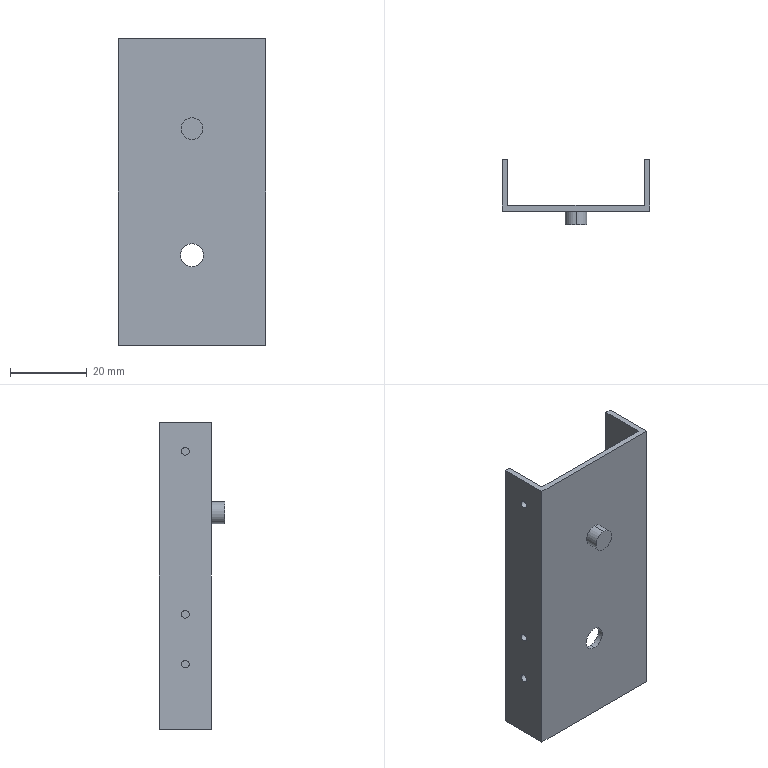Part | SolidWorks | features BaseBody 1 | 1 solid | 21 faces | box 38.6 x 17 x 80 mm | volume 7545 mm3 | plane 11 | cylinder 10 | commonest cylinder face diameters 2 x6 5.7 x2 6 x2
STEP:
#1=CARTESIAN_POINT('',(0.,-3.5,13.65));
#2=VERTEX_POINT('',#1);
#3=CARTESIAN_POINT('',(0.,-3.5,19.35));
#4=VERTEX_POINT('',#3);
#5=CARTESIAN_POINT('',(0.,-3.5,16.5));
#6=DIRECTION('',(0.,-1.,0.));
#7=DIRECTION('',(0.,0.,-1.));
#8=AXIS2_PLACEMENT_3D('',#5,#6,#7);
#9=CIRCLE('',#8,2.85);
#10=EDGE_CURVE('',#2,#4,#9,.T.);
#11=ORIENTED_EDGE('',*,*,#10,.F.);
#12=CARTESIAN_POINT('',(0.,0.,13.65));
#13=VERTEX_POINT('',#12);
#14=CARTESIAN_POINT('',(0.,-3.5,13.65));
#15=DIRECTION('',(0.,1.,0.));
#16=VECTOR('',#15,1000.);
#17=LINE('',#14,#16);
#18=EDGE_CURVE('',#2,#13,#17,.T.);
#19=ORIENTED_EDGE('',*,*,#18,.T.);
#20=CARTESIAN_POINT('',(0.,0.,19.35));
#21=VERTEX_POINT('',#20);
#22=CARTESIAN_POINT('',(0.,0.,16.5));
#23=DIRECTION('',(0.,-1.,0.));
#24=DIRECTION('',(0.,0.,1.));
#25=AXIS2_PLACEMENT_3D('',#22,#23,#24);
#26=CIRCLE('',#25,2.85);
#27=EDGE_CURVE('',#13,#21,#26,.T.);
#28=ORIENTED_EDGE('',*,*,#27,.T.);
#29=CARTESIAN_POINT('',(0.,-3.5,19.35));
#30=DIRECTION('',(0.,1.,0.));
#31=VECTOR('',#30,1000.);
#32=LINE('',#29,#31);
#33=EDGE_CURVE('',#4,#21,#32,.T.);
#34=ORIENTED_EDGE('',*,*,#33,.F.);
#35=EDGE_LOOP('',(#11,#19,#28,#34));
#36=FACE_OUTER_BOUND('',#35,.T.);
#37=CARTESIAN_POINT('',(0.,-3.5,16.5));
#38=DIRECTION('',(0.,1.,0.));
#39=DIRECTION('',(0.,0.,1.));
#40=AXIS2_PLACEMENT_3D('',#37,#38,#39);
#41=CYLINDRICAL_SURFACE('',#40,2.85);
#42=ADVANCED_FACE('',(#36),#41,.T.);
#43=CARTESIAN_POINT('',(-17.8,5.75,32.5));
#44=VERTEX_POINT('',#43);
#45=CARTESIAN_POINT('',(-17.8,7.75,32.5));
#46=VERTEX_POINT('',#45);
#47=CARTESIAN_POINT('',(-17.8,6.75,32.5));
#48=DIRECTION('',(1.,0.,0.));
#49=DIRECTION('',(0.,0.,1.));
#50=AXIS2_PLACEMENT_3D('',#47,#48,#49);
#51=CIRCLE('',#50,1.);
#52=EDGE_CURVE('',#44,#46,#51,.T.);
#53=ORIENTED_EDGE('',*,*,#52,.T.);
#54=CARTESIAN_POINT('',(-19.3,7.75,32.5));
#55=VERTEX_POINT('',#54);
#56=CARTESIAN_POINT('',(19.301,7.75,32.5));
#57=DIRECTION('',(-1.,0.,0.));
#58=VECTOR('',#57,1000.);
#59=LINE('',#56,#58);
#60=EDGE_CURVE('',#46,#55,#59,.T.);
#61=ORIENTED_EDGE('',*,*,#60,.T.);
#62=CARTESIAN_POINT('',(-19.3,5.75,32.5));
#63=VERTEX_POINT('',#62);
#64=CARTESIAN_POINT('',(-19.3,6.75,32.5));
#65=DIRECTION('',(-1.,0.,0.));
#66=DIRECTION('',(0.,-1.,0.));
#67=AXIS2_PLACEMENT_3D('',#64,#65,#66);
#68=CIRCLE('',#67,1.);
#69=EDGE_CURVE('',#55,#63,#68,.T.);
#70=ORIENTED_EDGE('',*,*,#69,.T.);
#71=CARTESIAN_POINT('',(19.301,5.75,32.5));
#72=DIRECTION('',(-1.,0.,0.));
#73=VECTOR('',#72,1000.);
#74=LINE('',#71,#73);
#75=EDGE_CURVE('',#44,#63,#74,.T.);
#76=ORIENTED_EDGE('',*,*,#75,.F.);
#77=EDGE_LOOP('',(#53,#61,#70,#76));
#78=FACE_OUTER_BOUND('',#77,.T.);
#79=CARTESIAN_POINT('',(19.301,6.75,32.5));
#80=DIRECTION('',(-1.,0.,0.));
#81=DIRECTION('',(0.,-1.,0.));
#82=AXIS2_PLACEMENT_3D('',#79,#80,#81);
#83=CYLINDRICAL_SURFACE('',#82,1.);
#84=ADVANCED_FACE('',(#78),#83,.F.);
#85=CARTESIAN_POINT('',(-17.8,5.75,-10.));
#86=VERTEX_POINT('',#85);
#87=CARTESIAN_POINT('',(-17.8,7.75,-10.));
#88=VERTEX_POINT('',#87);
#89=CARTESIAN_POINT('',(-17.8,6.75,-10.));
#90=DIRECTION('',(1.,0.,0.));
#91=DIRECTION('',(0.,0.,1.));
#92=AXIS2_PLACEMENT_3D('',#89,#90,#91);
#93=CIRCLE('',#92,1.);
#94=EDGE_CURVE('',#86,#88,#93,.T.);
#95=ORIENTED_EDGE('',*,*,#94,.T.);
#96=CARTESIAN_POINT('',(-19.3,7.75,-10.));
#97=VERTEX_POINT('',#96);
#98=CARTESIAN_POINT('',(19.301,7.75,-10.));
#99=DIRECTION('',(-1.,0.,0.));
#100=VECTOR('',#99,1000.);
#101=LINE('',#98,#100);
#102=EDGE_CURVE('',#88,#97,#101,.T.);
#103=ORIENTED_EDGE('',*,*,#102,.T.);
#104=CARTESIAN_POINT('',(-19.3,5.75,-10.));
#105=VERTEX_POINT('',#104);
#106=CARTESIAN_POINT('',(-19.3,6.75,-10.));
#107=DIRECTION('',(-1.,0.,0.));
#108=DIRECTION('',(0.,-1.,0.));
#109=AXIS2_PLACEMENT_3D('',#106,#107,#108);
#110=CIRCLE('',#109,1.);
#111=EDGE_CURVE('',#97,#105,#110,.T.);
#112=ORIENTED_EDGE('',*,*,#111,.T.);
#113=CARTESIAN_POINT('',(19.301,5.75,-10.));
#114=DIRECTION('',(-1.,0.,0.));
#115=VECTOR('',#114,1000.);
#116=LINE('',#113,#115);
#117=EDGE_CURVE('',#86,#105,#116,.T.);
#118=ORIENTED_EDGE('',*,*,#117,.F.);
#119=EDGE_LOOP('',(#95,#103,#112,#118));
#120=FACE_OUTER_BOUND('',#119,.T.);
#121=CARTESIAN_POINT('',(19.301,6.75,-10.));
#122=DIRECTION('',(-1.,0.,0.));
#123=DIRECTION('',(0.,-1.,0.));
#124=AXIS2_PLACEMENT_3D('',#121,#122,#123);
#125=CYLINDRICAL_SURFACE('',#124,1.);
#126=ADVANCED_FACE('',(#120),#125,.F.);
#127=CARTESIAN_POINT('',(-17.8,5.75,-23.));
#128=VERTEX_POINT('',#127);
#129=CARTESIAN_POINT('',(-17.8,7.75,-23.));
#130=VERTEX_POINT('',#129);
#131=CARTESIAN_POINT('',(-17.8,6.75,-23.));
#132=DIRECTION('',(1.,0.,0.));
#133=DIRECTION('',(0.,0.,1.));
#134=AXIS2_PLACEMENT_3D('',#131,#132,#133);
#135=CIRCLE('',#134,1.);
#136=EDGE_CURVE('',#128,#130,#135,.T.);
#137=ORIENTED_EDGE('',*,*,#136,.T.);
#138=CARTESIAN_POINT('',(-19.3,7.75,-23.));
#139=VERTEX_POINT('',#138);
#140=CARTESIAN_POINT('',(19.301,7.75,-23.));
#141=DIRECTION('',(-1.,0.,0.));
#142=VECTOR('',#141,1000.);
#143=LINE('',#140,#142);
#144=EDGE_CURVE('',#130,#139,#143,.T.);
#145=ORIENTED_EDGE('',*,*,#144,.T.);
#146=CARTESIAN_POINT('',(-19.3,5.75,-23.));
#147=VERTEX_POINT('',#146);
#148=CARTESIAN_POINT('',(-19.3,6.75,-23.));
#149=DIRECTION('',(-1.,0.,0.));
#150=DIRECTION('',(0.,-1.,0.));
#151=AXIS2_PLACEMENT_3D('',#148,#149,#150);
#152=CIRCLE('',#151,1.);
#153=EDGE_CURVE('',#139,#147,#152,.T.);
#154=ORIENTED_EDGE('',*,*,#153,.T.);
#155=CARTESIAN_POINT('',(19.301,5.75,-23.));
#156=DIRECTION('',(-1.,0.,0.));
#157=VECTOR('',#156,1000.);
#158=LINE('',#155,#157);
#159=EDGE_CURVE('',#128,#147,#158,.T.);
#160=ORIENTED_EDGE('',*,*,#159,.F.);
#161=EDGE_LOOP('',(#137,#145,#154,#160));
#162=FACE_OUTER_BOUND('',#161,.T.);
#163=CARTESIAN_POINT('',(19.301,6.75,-23.));
#164=DIRECTION('',(-1.,0.,0.));
#165=DIRECTION('',(0.,-1.,0.));
#166=AXIS2_PLACEMENT_3D('',#163,#164,#165);
#167=CYLINDRICAL_SURFACE('',#166,1.);
#168=ADVANCED_FACE('',(#162),#167,.F.);
#169=CARTESIAN_POINT('',(0.,1.5,-13.5));
#170=VERTEX_POINT('',#169);
#171=CARTESIAN_POINT('',(0.,1.5,-19.5));
#172=VERTEX_POINT('',#171);
#173=CARTESIAN_POINT('',(0.,1.5,-16.5));
#174=DIRECTION('',(0.,-1.,0.));
#175=DIRECTION('',(0.,0.,-1.));
#176=AXIS2_PLACEMENT_3D('',#173,#174,#175);
#177=CIRCLE('',#176,3.);
#178=EDGE_CURVE('',#170,#172,#177,.T.);
#179=ORIENTED_EDGE('',*,*,#178,.F.);
#180=CARTESIAN_POINT('',(0.,0.,-13.5));
#181=VERTEX_POINT('',#180);
#182=CARTESIAN_POINT('',(0.,13.5,-13.5));
#183=DIRECTION('',(0.,-1.,0.));
#184=VECTOR('',#183,1000.);
#185=LINE('',#182,#184);
#186=EDGE_CURVE('',#170,#181,#185,.T.);
#187=ORIENTED_EDGE('',*,*,#186,.T.);
#188=CARTESIAN_POINT('',(0.,0.,-19.5));
#189=VERTEX_POINT('',#188);
#190=CARTESIAN_POINT('',(0.,0.,-16.5));
#191=DIRECTION('',(0.,-1.,0.));
#192=DIRECTION('',(0.,0.,-1.));
#193=AXIS2_PLACEMENT_3D('',#190,#191,#192);
#194=CIRCLE('',#193,3.);
#195=EDGE_CURVE('',#181,#189,#194,.T.);
#196=ORIENTED_EDGE('',*,*,#195,.T.);
#197=CARTESIAN_POINT('',(0.,13.5,-19.5));
#198=DIRECTION('',(0.,-1.,0.));
#199=VECTOR('',#198,1000.);
#200=LINE('',#197,#199);
#201=EDGE_CURVE('',#172,#189,#200,.T.);
#202=ORIENTED_EDGE('',*,*,#201,.F.);
#203=EDGE_LOOP('',(#179,#187,#196,#202));
#204=FACE_OUTER_BOUND('',#203,.T.);
#205=CARTESIAN_POINT('',(0.,13.5,-16.5));
#206=DIRECTION('',(0.,-1.,0.));
#207=DIRECTION('',(0.,0.,-1.));
#208=AXIS2_PLACEMENT_3D('',#205,#206,#207);
#209=CYLINDRICAL_SURFACE('',#208,3.);
#210=ADVANCED_FACE('',(#204),#209,.F.);
#211=CARTESIAN_POINT('',(-17.8,13.5,-40.));
#212=VERTEX_POINT('',#211);
#213=CARTESIAN_POINT('',(-19.3,13.5,-40.));
#214=VERTEX_POINT('',#213);
#215=CARTESIAN_POINT('',(-19.3,13.5,-40.));
#216=DIRECTION('',(-1.,0.,0.));
#217=VECTOR('',#216,1000.);
#218=LINE('',#215,#217);
#219=EDGE_CURVE('',#212,#214,#218,.T.);
#220=ORIENTED_EDGE('',*,*,#219,.T.);
#221=CARTESIAN_POINT('',(-19.3,13.5,40.));
#222=VERTEX_POINT('',#221);
#223=CARTESIAN_POINT('',(-19.3,13.5,40.));
#224=DIRECTION('',(0.,0.,-1.));
#225=VECTOR('',#224,1000.);
#226=LINE('',#223,#225);
#227=EDGE_CURVE('',#222,#214,#226,.T.);
#228=ORIENTED_EDGE('',*,*,#227,.F.);
#229=CARTESIAN_POINT('',(-17.8,13.5,40.));
#230=VERTEX_POINT('',#229);
#231=CARTESIAN_POINT('',(-19.3,13.5,40.));
#232=DIRECTION('',(-1.,0.,0.));
#233=VECTOR('',#232,1000.);
#234=LINE('',#231,#233);
#235=EDGE_CURVE('',#230,#222,#234,.T.);
#236=ORIENTED_EDGE('',*,*,#235,.F.);
#237=CARTESIAN_POINT('',(-17.8,13.5,40.));
#238=DIRECTION('',(0.,0.,-1.));
#239=VECTOR('',#238,1000.);
#240=LINE('',#237,#239);
#241=EDGE_CURVE('',#230,#212,#240,.T.);
#242=ORIENTED_EDGE('',*,*,#241,.T.);
#243=EDGE_LOOP('',(#220,#228,#236,#242));
#244=FACE_OUTER_BOUND('',#243,.T.);
#245=CARTESIAN_POINT('',(-19.3,13.5,40.));
#246=DIRECTION('',(0.,-1.,0.));
#247=DIRECTION('',(0.,0.,-1.));
#248=AXIS2_PLACEMENT_3D('',#245,#246,#247);
#249=PLANE('',#248);
#250=ADVANCED_FACE('',(#244),#249,.F.);
#251=CARTESIAN_POINT('',(-19.3,6.75,32.5));
#252=DIRECTION('',(-1.,0.,0.));
#253=DIRECTION('',(0.,-1.,0.));
#254=AXIS2_PLACEMENT_3D('',#251,#252,#253);
#255=CIRCLE('',#254,1.);
#256=EDGE_CURVE('',#63,#55,#255,.T.);
#257=ORIENTED_EDGE('',*,*,#256,.F.);
#258=ORIENTED_EDGE('',*,*,#69,.F.);
#259=EDGE_LOOP('',(#257,#258));
#260=FACE_BOUND('',#259,.T.);
#261=CARTESIAN_POINT('',(-19.3,6.75,-10.));
#262=DIRECTION('',(-1.,0.,0.));
#263=DIRECTION('',(0.,-1.,0.));
#264=AXIS2_PLACEMENT_3D('',#261,#262,#263);
#265=CIRCLE('',#264,1.);
#266=EDGE_CURVE('',#105,#97,#265,.T.);
#267=ORIENTED_EDGE('',*,*,#266,.F.);
#268=ORIENTED_EDGE('',*,*,#111,.F.);
#269=EDGE_LOOP('',(#267,#268));
#270=FACE_BOUND('',#269,.T.);
#271=CARTESIAN_POINT('',(-19.3,6.75,-23.));
#272=DIRECTION('',(-1.,0.,0.));
#273=DIRECTION('',(0.,-1.,0.));
#274=AXIS2_PLACEMENT_3D('',#271,#272,#273);
#275=CIRCLE('',#274,1.);
#276=EDGE_CURVE('',#147,#139,#275,.T.);
#277=ORIENTED_EDGE('',*,*,#276,.F.);
#278=ORIENTED_EDGE('',*,*,#153,.F.);
#279=EDGE_LOOP('',(#277,#278));
#280=FACE_BOUND('',#279,.T.);
#281=CARTESIAN_POINT('',(-19.3,0.,-40.));
#282=VERTEX_POINT('',#281);
#283=CARTESIAN_POINT('',(-19.3,13.5,-40.));
#284=DIRECTION('',(0.,-1.,0.));
#285=VECTOR('',#284,1000.);
#286=LINE('',#283,#285);
#287=EDGE_CURVE('',#214,#282,#286,.T.);
#288=ORIENTED_EDGE('',*,*,#287,.T.);
#289=CARTESIAN_POINT('',(-19.3,0.,40.));
#290=VERTEX_POINT('',#289);
#291=CARTESIAN_POINT('',(-19.3,0.,40.));
#292=DIRECTION('',(0.,0.,-1.));
#293=VECTOR('',#292,1000.);
#294=LINE('',#291,#293);
#295=EDGE_CURVE('',#290,#282,#294,.T.);
#296=ORIENTED_EDGE('',*,*,#295,.F.);
#297=CARTESIAN_POINT('',(-19.3,13.5,40.));
#298=DIRECTION('',(0.,-1.,0.));
#299=VECTOR('',#298,1000.);
#300=LINE('',#297,#299);
#301=EDGE_CURVE('',#222,#290,#300,.T.);
#302=ORIENTED_EDGE('',*,*,#301,.F.);
#303=ORIENTED_EDGE('',*,*,#227,.T.);
#304=EDGE_LOOP('',(#288,#296,#302,#303));
#305=FACE_OUTER_BOUND('',#304,.T.);
#306=CARTESIAN_POINT('',(-19.3,13.5,40.));
#307=DIRECTION('',(1.,0.,0.));
#308=DIRECTION('',(0.,1.,0.));
#309=AXIS2_PLACEMENT_3D('',#306,#307,#308);
#310=PLANE('',#309);
#311=ADVANCED_FACE('',(#260,#270,#280,#305),#310,.F.);
#312=CARTESIAN_POINT('',(0.,0.,16.5));
#313=DIRECTION('',(0.,-1.,0.));
#314=DIRECTION('',(0.,0.,1.));
#315=AXIS2_PLACEMENT_3D('',#312,#313,#314);
#316=CIRCLE('',#315,2.85);
#317=EDGE_CURVE('',#21,#13,#316,.T.);
#318=ORIENTED_EDGE('',*,*,#317,.F.);
#319=ORIENTED_EDGE('',*,*,#27,.F.);
#320=EDGE_LOOP('',(#318,#319));
#321=FACE_BOUND('',#320,.T.);
#322=CARTESIAN_POINT('',(0.,0.,-16.5));
#323=DIRECTION('',(0.,-1.,0.));
#324=DIRECTION('',(0.,0.,-1.));
#325=AXIS2_PLACEMENT_3D('',#322,#323,#324);
#326=CIRCLE('',#325,3.);
#327=EDGE_CURVE('',#189,#181,#326,.T.);
#328=ORIENTED_EDGE('',*,*,#327,.F.);
#329=ORIENTED_EDGE('',*,*,#195,.F.);
#330=EDGE_LOOP('',(#328,#329));
#331=FACE_BOUND('',#330,.T.);
#332=CARTESIAN_POINT('',(19.3,0.,-40.));
#333=VERTEX_POINT('',#332);
#334=CARTESIAN_POINT('',(-19.3,0.,-40.));
#335=DIRECTION('',(1.,0.,0.));
#336=VECTOR('',#335,1000.);
#337=LINE('',#334,#336);
#338=EDGE_CURVE('',#282,#333,#337,.T.);
#339=ORIENTED_EDGE('',*,*,#338,.T.);
#340=CARTESIAN_POINT('',(19.3,0.,40.));
#341=VERTEX_POINT('',#340);
#342=CARTESIAN_POINT('',(19.3,0.,40.));
#343=DIRECTION('',(0.,0.,-1.));
#344=VECTOR('',#343,1000.);
#345=LINE('',#342,#344);
#346=EDGE_CURVE('',#341,#333,#345,.T.);
#347=ORIENTED_EDGE('',*,*,#346,.F.);
#348=CARTESIAN_POINT('',(-19.3,0.,40.));
#349=DIRECTION('',(1.,0.,0.));
#350=VECTOR('',#349,1000.);
#351=LINE('',#348,#350);
#352=EDGE_CURVE('',#290,#341,#351,.T.);
#353=ORIENTED_EDGE('',*,*,#352,.F.);
#354=ORIENTED_EDGE('',*,*,#295,.T.);
#355=EDGE_LOOP('',(#339,#347,#353,#354));
#356=FACE_OUTER_BOUND('',#355,.T.);
#357=CARTESIAN_POINT('',(-19.3,0.,40.));
#358=DIRECTION('',(0.,1.,0.));
#359=DIRECTION('',(0.,0.,1.));
#360=AXIS2_PLACEMENT_3D('',#357,#358,#359);
#361=PLANE('',#360);
#362=ADVANCED_FACE('',(#321,#331,#356),#361,.F.);
#363=CARTESIAN_POINT('',(19.3,13.5,-40.));
#364=VERTEX_POINT('',#363);
#365=CARTESIAN_POINT('',(19.3,0.,-40.));
#366=DIRECTION('',(0.,1.,0.));
#367=VECTOR('',#366,1000.);
#368=LINE('',#365,#367);
#369=EDGE_CURVE('',#333,#364,#368,.T.);
#370=ORIENTED_EDGE('',*,*,#369,.T.);
#371=CARTESIAN_POINT('',(19.3,13.5,40.));
#372=VERTEX_POINT('',#371);
#373=CARTESIAN_POINT('',(19.3,13.5,40.));
#374=DIRECTION('',(0.,0.,-1.));
#375=VECTOR('',#374,1000.);
#376=LINE('',#373,#375);
#377=EDGE_CURVE('',#372,#364,#376,.T.);
#378=ORIENTED_EDGE('',*,*,#377,.F.);
#379=CARTESIAN_POINT('',(19.3,0.,40.));
#380=DIRECTION('',(0.,1.,0.));
#381=VECTOR('',#380,1000.);
#382=LINE('',#379,#381);
#383=EDGE_CURVE('',#341,#372,#382,.T.);
#384=ORIENTED_EDGE('',*,*,#383,.F.);
#385=ORIENTED_EDGE('',*,*,#346,.T.);
#386=EDGE_LOOP('',(#370,#378,#384,#385));
#387=FACE_OUTER_BOUND('',#386,.T.);
#388=CARTESIAN_POINT('',(19.3,0.,40.));
#389=DIRECTION('',(-1.,0.,0.));
#390=DIRECTION('',(0.,-1.,0.));
#391=AXIS2_PLACEMENT_3D('',#388,#389,#390);
#392=PLANE('',#391);
#393=ADVANCED_FACE('',(#387),#392,.F.);
#394=CARTESIAN_POINT('',(17.8,13.5,-40.));
#395=VERTEX_POINT('',#394);
#396=CARTESIAN_POINT('',(17.8,13.5,-40.));
#397=DIRECTION('',(-1.,0.,0.));
#398=VECTOR('',#397,1000.);
#399=LINE('',#396,#398);
#400=EDGE_CURVE('',#364,#395,#399,.T.);
#401=ORIENTED_EDGE('',*,*,#400,.T.);
#402=CARTESIAN_POINT('',(17.8,13.5,40.));
#403=VERTEX_POINT('',#402);
#404=CARTESIAN_POINT('',(17.8,13.5,40.));
#405=DIRECTION('',(0.,0.,-1.));
#406=VECTOR('',#405,1000.);
#407=LINE('',#404,#406);
#408=EDGE_CURVE('',#403,#395,#407,.T.);
#409=ORIENTED_EDGE('',*,*,#408,.F.);
#410=CARTESIAN_POINT('',(17.8,13.5,40.));
#411=DIRECTION('',(-1.,0.,0.));
#412=VECTOR('',#411,1000.);
#413=LINE('',#410,#412);
#414=EDGE_CURVE('',#372,#403,#413,.T.);
#415=ORIENTED_EDGE('',*,*,#414,.F.);
#416=ORIENTED_EDGE('',*,*,#377,.T.);
#417=EDGE_LOOP('',(#401,#409,#415,#416));
#418=FACE_OUTER_BOUND('',#417,.T.);
#419=CARTESIAN_POINT('',(17.8,13.5,40.));
#420=DIRECTION('',(0.,-1.,0.));
#421=DIRECTION('',(0.,0.,-1.));
#422=AXIS2_PLACEMENT_3D('',#419,#420,#421);
#423=PLANE('',#422);
#424=ADVANCED_FACE('',(#418),#423,.F.);
#425=CARTESIAN_POINT('',(17.8,1.5,-40.));
#426=VERTEX_POINT('',#425);
#427=CARTESIAN_POINT('',(17.8,1.5,-40.));
#428=DIRECTION('',(0.,-1.,0.));
#429=VECTOR('',#428,1000.);
#430=LINE('',#427,#429);
#431=EDGE_CURVE('',#395,#426,#430,.T.);
#432=ORIENTED_EDGE('',*,*,#431,.T.);
#433=CARTESIAN_POINT('',(17.8,1.5,40.));
#434=VERTEX_POINT('',#433);
#435=CARTESIAN_POINT('',(17.8,1.5,40.));
#436=DIRECTION('',(0.,0.,-1.));
#437=VECTOR('',#436,1000.);
#438=LINE('',#435,#437);
#439=EDGE_CURVE('',#434,#426,#438,.T.);
#440=ORIENTED_EDGE('',*,*,#439,.F.);
#441=CARTESIAN_POINT('',(17.8,1.5,40.));
#442=DIRECTION('',(0.,-1.,0.));
#443=VECTOR('',#442,1000.);
#444=LINE('',#441,#443);
#445=EDGE_CURVE('',#403,#434,#444,.T.);
#446=ORIENTED_EDGE('',*,*,#445,.F.);
#447=ORIENTED_EDGE('',*,*,#408,.T.);
#448=EDGE_LOOP('',(#432,#440,#446,#447));
#449=FACE_OUTER_BOUND('',#448,.T.);
#450=CARTESIAN_POINT('',(17.8,1.5,40.));
#451=DIRECTION('',(1.,0.,0.));
#452=DIRECTION('',(0.,0.,-1.));
#453=AXIS2_PLACEMENT_3D('',#450,#451,#452);
#454=PLANE('',#453);
#455=ADVANCED_FACE('',(#449),#454,.F.);
#456=CARTESIAN_POINT('',(0.,1.5,-16.5));
#457=DIRECTION('',(0.,-1.,0.));
#458=DIRECTION('',(0.,0.,-1.));
#459=AXIS2_PLACEMENT_3D('',#456,#457,#458);
#460=CIRCLE('',#459,3.);
#461=EDGE_CURVE('',#172,#170,#460,.T.);
#462=ORIENTED_EDGE('',*,*,#461,.T.);
#463=ORIENTED_EDGE('',*,*,#178,.T.);
#464=EDGE_LOOP('',(#462,#463));
#465=FACE_BOUND('',#464,.T.);
#466=CARTESIAN_POINT('',(-17.8,1.5,-40.));
#467=VERTEX_POINT('',#466);
#468=CARTESIAN_POINT('',(-17.8,1.5,-40.));
#469=DIRECTION('',(-1.,0.,0.));
#470=VECTOR('',#469,1000.);
#471=LINE('',#468,#470);
#472=EDGE_CURVE('',#426,#467,#471,.T.);
#473=ORIENTED_EDGE('',*,*,#472,.T.);
#474=CARTESIAN_POINT('',(-17.8,1.5,40.));
#475=VERTEX_POINT('',#474);
#476=CARTESIAN_POINT('',(-17.8,1.5,40.));
#477=DIRECTION('',(0.,0.,-1.));
#478=VECTOR('',#477,1000.);
#479=LINE('',#476,#478);
#480=EDGE_CURVE('',#475,#467,#479,.T.);
#481=ORIENTED_EDGE('',*,*,#480,.F.);
#482=CARTESIAN_POINT('',(-17.8,1.5,40.));
#483=DIRECTION('',(-1.,0.,0.));
#484=VECTOR('',#483,1000.);
#485=LINE('',#482,#484);
#486=EDGE_CURVE('',#434,#475,#485,.T.);
#487=ORIENTED_EDGE('',*,*,#486,.F.);
#488=ORIENTED_EDGE('',*,*,#439,.T.);
#489=EDGE_LOOP('',(#473,#481,#487,#488));
#490=FACE_OUTER_BOUND('',#489,.T.);
#491=CARTESIAN_POINT('',(-17.8,1.5,40.));
#492=DIRECTION('',(0.,-1.,0.));
#493=DIRECTION('',(0.,0.,-1.));
#494=AXIS2_PLACEMENT_3D('',#491,#492,#493);
#495=PLANE('',#494);
#496=ADVANCED_FACE('',(#465,#490),#495,.F.);
#497=ORIENTED_EDGE('',*,*,#52,.F.);
#498=CARTESIAN_POINT('',(-17.8,6.75,32.5));
#499=DIRECTION('',(1.,0.,0.));
#500=DIRECTION('',(0.,0.,1.));
#501=AXIS2_PLACEMENT_3D('',#498,#499,#500);
#502=CIRCLE('',#501,1.);
#503=EDGE_CURVE('',#46,#44,#502,.T.);
#504=ORIENTED_EDGE('',*,*,#503,.F.);
#505=EDGE_LOOP('',(#497,#504));
#506=FACE_BOUND('',#505,.T.);
#507=ORIENTED_EDGE('',*,*,#94,.F.);
#508=CARTESIAN_POINT('',(-17.8,6.75,-10.));
#509=DIRECTION('',(1.,0.,0.));
#510=DIRECTION('',(0.,0.,1.));
#511=AXIS2_PLACEMENT_3D('',#508,#509,#510);
#512=CIRCLE('',#511,1.);
#513=EDGE_CURVE('',#88,#86,#512,.T.);
#514=ORIENTED_EDGE('',*,*,#513,.F.);
#515=EDGE_LOOP('',(#507,#514));
#516=FACE_BOUND('',#515,.T.);
#517=ORIENTED_EDGE('',*,*,#136,.F.);
#518=CARTESIAN_POINT('',(-17.8,6.75,-23.));
#519=DIRECTION('',(1.,0.,0.));
#520=DIRECTION('',(0.,0.,1.));
#521=AXIS2_PLACEMENT_3D('',#518,#519,#520);
#522=CIRCLE('',#521,1.);
#523=EDGE_CURVE('',#130,#128,#522,.T.);
#524=ORIENTED_EDGE('',*,*,#523,.F.);
#525=EDGE_LOOP('',(#517,#524));
#526=FACE_BOUND('',#525,.T.);
#527=CARTESIAN_POINT('',(-17.8,13.5,-40.));
#528=DIRECTION('',(0.,1.,0.));
#529=VECTOR('',#528,1000.);
#530=LINE('',#527,#529);
#531=EDGE_CURVE('',#467,#212,#530,.T.);
#532=ORIENTED_EDGE('',*,*,#531,.T.);
#533=ORIENTED_EDGE('',*,*,#241,.F.);
#534=CARTESIAN_POINT('',(-17.8,13.5,40.));
#535=DIRECTION('',(0.,1.,0.));
#536=VECTOR('',#535,1000.);
#537=LINE('',#534,#536);
#538=EDGE_CURVE('',#475,#230,#537,.T.);
#539=ORIENTED_EDGE('',*,*,#538,.F.);
#540=ORIENTED_EDGE('',*,*,#480,.T.);
#541=EDGE_LOOP('',(#532,#533,#539,#540));
#542=FACE_OUTER_BOUND('',#541,.T.);
#543=CARTESIAN_POINT('',(-17.8,13.5,40.));
#544=DIRECTION('',(-1.,0.,0.));
#545=DIRECTION('',(0.,0.,1.));
#546=AXIS2_PLACEMENT_3D('',#543,#544,#545);
#547=PLANE('',#546);
#548=ADVANCED_FACE('',(#506,#516,#526,#542),#547,.F.);
#549=ORIENTED_EDGE('',*,*,#235,.T.);
#550=ORIENTED_EDGE('',*,*,#301,.T.);
#551=ORIENTED_EDGE('',*,*,#352,.T.);
#552=ORIENTED_EDGE('',*,*,#383,.T.);
#553=ORIENTED_EDGE('',*,*,#414,.T.);
#554=ORIENTED_EDGE('',*,*,#445,.T.);
#555=ORIENTED_EDGE('',*,*,#486,.T.);
#556=ORIENTED_EDGE('',*,*,#538,.T.);
#557=EDGE_LOOP('',(#549,#550,#551,#552,#553,#554,#555,#556));
#558=FACE_OUTER_BOUND('',#557,.T.);
#559=CARTESIAN_POINT('',(0.,0.,40.));
#560=DIRECTION('',(0.,0.,-1.));
#561=DIRECTION('',(-1.,0.,0.));
#562=AXIS2_PLACEMENT_3D('',#559,#560,#561);
#563=PLANE('',#562);
#564=ADVANCED_FACE('',(#558),#563,.F.);
#565=ORIENTED_EDGE('',*,*,#219,.F.);
#566=ORIENTED_EDGE('',*,*,#531,.F.);
#567=ORIENTED_EDGE('',*,*,#472,.F.);
#568=ORIENTED_EDGE('',*,*,#431,.F.);
#569=ORIENTED_EDGE('',*,*,#400,.F.);
#570=ORIENTED_EDGE('',*,*,#369,.F.);
#571=ORIENTED_EDGE('',*,*,#338,.F.);
#572=ORIENTED_EDGE('',*,*,#287,.F.);
#573=EDGE_LOOP('',(#565,#566,#567,#568,#569,#570,#571,#572));
#574=FACE_OUTER_BOUND('',#573,.T.);
#575=CARTESIAN_POINT('',(0.,0.,-40.));
#576=DIRECTION('',(0.,0.,-1.));
#577=DIRECTION('',(-1.,0.,0.));
#578=AXIS2_PLACEMENT_3D('',#575,#576,#577);
#579=PLANE('',#578);
#580=ADVANCED_FACE('',(#574),#579,.T.);
#581=ORIENTED_EDGE('',*,*,#186,.F.);
#582=ORIENTED_EDGE('',*,*,#461,.F.);
#583=ORIENTED_EDGE('',*,*,#201,.T.);
#584=ORIENTED_EDGE('',*,*,#327,.T.);
#585=EDGE_LOOP('',(#581,#582,#583,#584));
#586=FACE_OUTER_BOUND('',#585,.T.);
#587=CARTESIAN_POINT('',(0.,13.5,-16.5));
#588=DIRECTION('',(0.,-1.,0.));
#589=DIRECTION('',(0.,0.,-1.));
#590=AXIS2_PLACEMENT_3D('',#587,#588,#589);
#591=CYLINDRICAL_SURFACE('',#590,3.);
#592=ADVANCED_FACE('',(#586),#591,.F.);
#593=ORIENTED_EDGE('',*,*,#144,.F.);
#594=ORIENTED_EDGE('',*,*,#523,.T.);
#595=ORIENTED_EDGE('',*,*,#159,.T.);
#596=ORIENTED_EDGE('',*,*,#276,.T.);
#597=EDGE_LOOP('',(#593,#594,#595,#596));
#598=FACE_OUTER_BOUND('',#597,.T.);
#599=CARTESIAN_POINT('',(19.301,6.75,-23.));
#600=DIRECTION('',(-1.,0.,0.));
#601=DIRECTION('',(0.,-1.,0.));
#602=AXIS2_PLACEMENT_3D('',#599,#600,#601);
#603=CYLINDRICAL_SURFACE('',#602,1.);
#604=ADVANCED_FACE('',(#598),#603,.F.);
#605=ORIENTED_EDGE('',*,*,#102,.F.);
#606=ORIENTED_EDGE('',*,*,#513,.T.);
#607=ORIENTED_EDGE('',*,*,#117,.T.);
#608=ORIENTED_EDGE('',*,*,#266,.T.);
#609=EDGE_LOOP('',(#605,#606,#607,#608));
#610=FACE_OUTER_BOUND('',#609,.T.);
#611=CARTESIAN_POINT('',(19.301,6.75,-10.));
#612=DIRECTION('',(-1.,0.,0.));
#613=DIRECTION('',(0.,-1.,0.));
#614=AXIS2_PLACEMENT_3D('',#611,#612,#613);
#615=CYLINDRICAL_SURFACE('',#614,1.);
#616=ADVANCED_FACE('',(#610),#615,.F.);
#617=ORIENTED_EDGE('',*,*,#60,.F.);
#618=ORIENTED_EDGE('',*,*,#503,.T.);
#619=ORIENTED_EDGE('',*,*,#75,.T.);
#620=ORIENTED_EDGE('',*,*,#256,.T.);
#621=EDGE_LOOP('',(#617,#618,#619,#620));
#622=FACE_OUTER_BOUND('',#621,.T.);
#623=CARTESIAN_POINT('',(19.301,6.75,32.5));
#624=DIRECTION('',(-1.,0.,0.));
#625=DIRECTION('',(0.,-1.,0.));
#626=AXIS2_PLACEMENT_3D('',#623,#624,#625);
#627=CYLINDRICAL_SURFACE('',#626,1.);
#628=ADVANCED_FACE('',(#622),#627,.F.);
#629=ORIENTED_EDGE('',*,*,#18,.F.);
#630=CARTESIAN_POINT('',(0.,-3.5,16.5));
#631=DIRECTION('',(0.,-1.,0.));
#632=DIRECTION('',(0.,0.,-1.));
#633=AXIS2_PLACEMENT_3D('',#630,#631,#632);
#634=CIRCLE('',#633,2.85);
#635=EDGE_CURVE('',#4,#2,#634,.T.);
#636=ORIENTED_EDGE('',*,*,#635,.F.);
#637=ORIENTED_EDGE('',*,*,#33,.T.);
#638=ORIENTED_EDGE('',*,*,#317,.T.);
#639=EDGE_LOOP('',(#629,#636,#637,#638));
#640=FACE_OUTER_BOUND('',#639,.T.);
#641=CARTESIAN_POINT('',(0.,-3.5,16.5));
#642=DIRECTION('',(0.,1.,0.));
#643=DIRECTION('',(0.,0.,1.));
#644=AXIS2_PLACEMENT_3D('',#641,#642,#643);
#645=CYLINDRICAL_SURFACE('',#644,2.85);
#646=ADVANCED_FACE('',(#640),#645,.T.);
#647=ORIENTED_EDGE('',*,*,#635,.T.);
#648=ORIENTED_EDGE('',*,*,#10,.T.);
#649=EDGE_LOOP('',(#647,#648));
#650=FACE_OUTER_BOUND('',#649,.T.);
#651=CARTESIAN_POINT('',(0.,-3.5,16.5));
#652=DIRECTION('',(0.,-1.,0.));
#653=DIRECTION('',(0.,0.,-1.));
#654=AXIS2_PLACEMENT_3D('',#651,#652,#653);
#655=PLANE('',#654);
#656=ADVANCED_FACE('',(#650),#655,.T.);
#657=CLOSED_SHELL('',(#42,#84,#126,#168,#210,#250,#311,#362,#393,#424,#455,#496,#548,#564,#580,#592,#604,#616,#628,#646,#656));
#658=MANIFOLD_SOLID_BREP('',#657);
#659=CARTESIAN_POINT('',(0.,0.,0.));
#660=DIRECTION('',(0.,0.,1.));
#661=DIRECTION('',(1.,0.,0.));
#662=AXIS2_PLACEMENT_3D('',#659,#660,#661);
#663=(LENGTH_UNIT()NAMED_UNIT(*)SI_UNIT(.MILLI.,.METRE.));
#664=UNCERTAINTY_MEASURE_WITH_UNIT(LENGTH_MEASURE(0.00001),#663,'','');
#665=(NAMED_UNIT(*)PLANE_ANGLE_UNIT()SI_UNIT($,.RADIAN.));
#666=(NAMED_UNIT(*)SI_UNIT($,.STERADIAN.)SOLID_ANGLE_UNIT());
#667=(GEOMETRIC_REPRESENTATION_CONTEXT(3)GLOBAL_UNCERTAINTY_ASSIGNED_CONTEXT((#664))GLOBAL_UNIT_ASSIGNED_CONTEXT((#663,#665,#666))REPRESENTATION_CONTEXT('',''));
#668=ADVANCED_BREP_SHAPE_REPRESENTATION('',(#658,#662),#667);